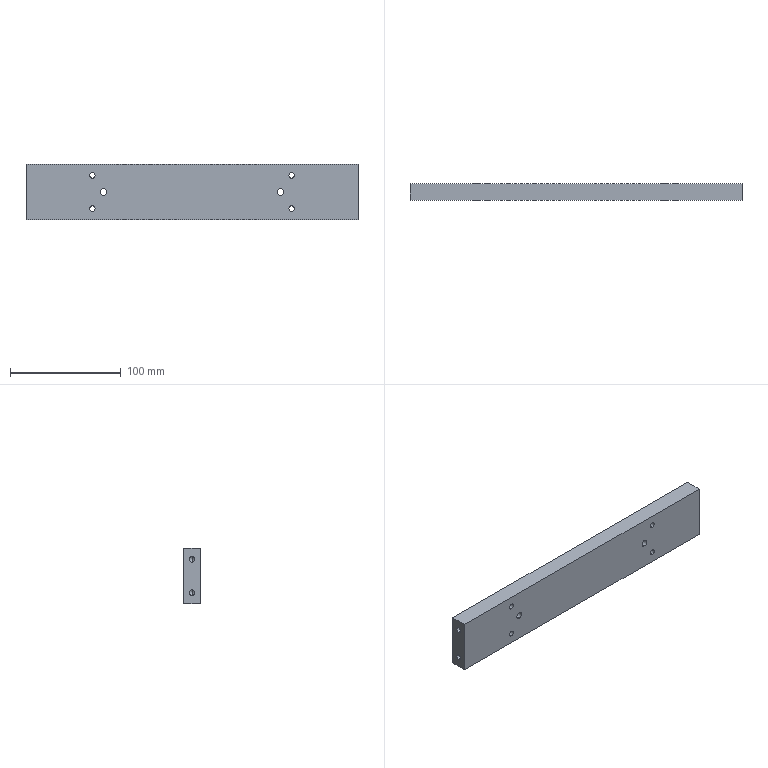Part | STEP file | A14-018 | 1 solid | 46 faces | box 300 x 15 x 50 mm | volume 221576 mm3 | cylinder 24 | cone 16 | plane 6 | commonest cylinder face diameters 5 x16 3.3 x4 6 x4